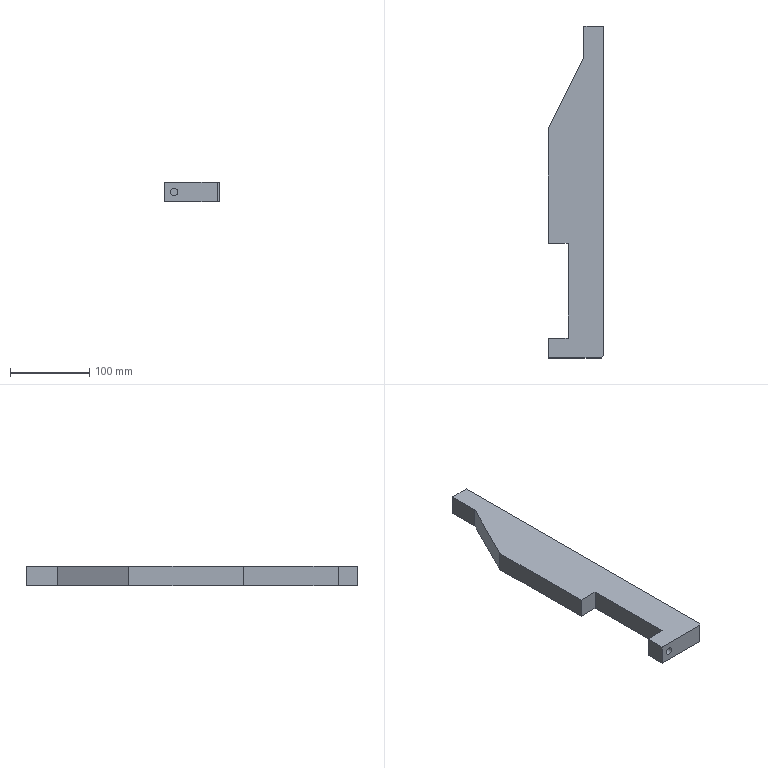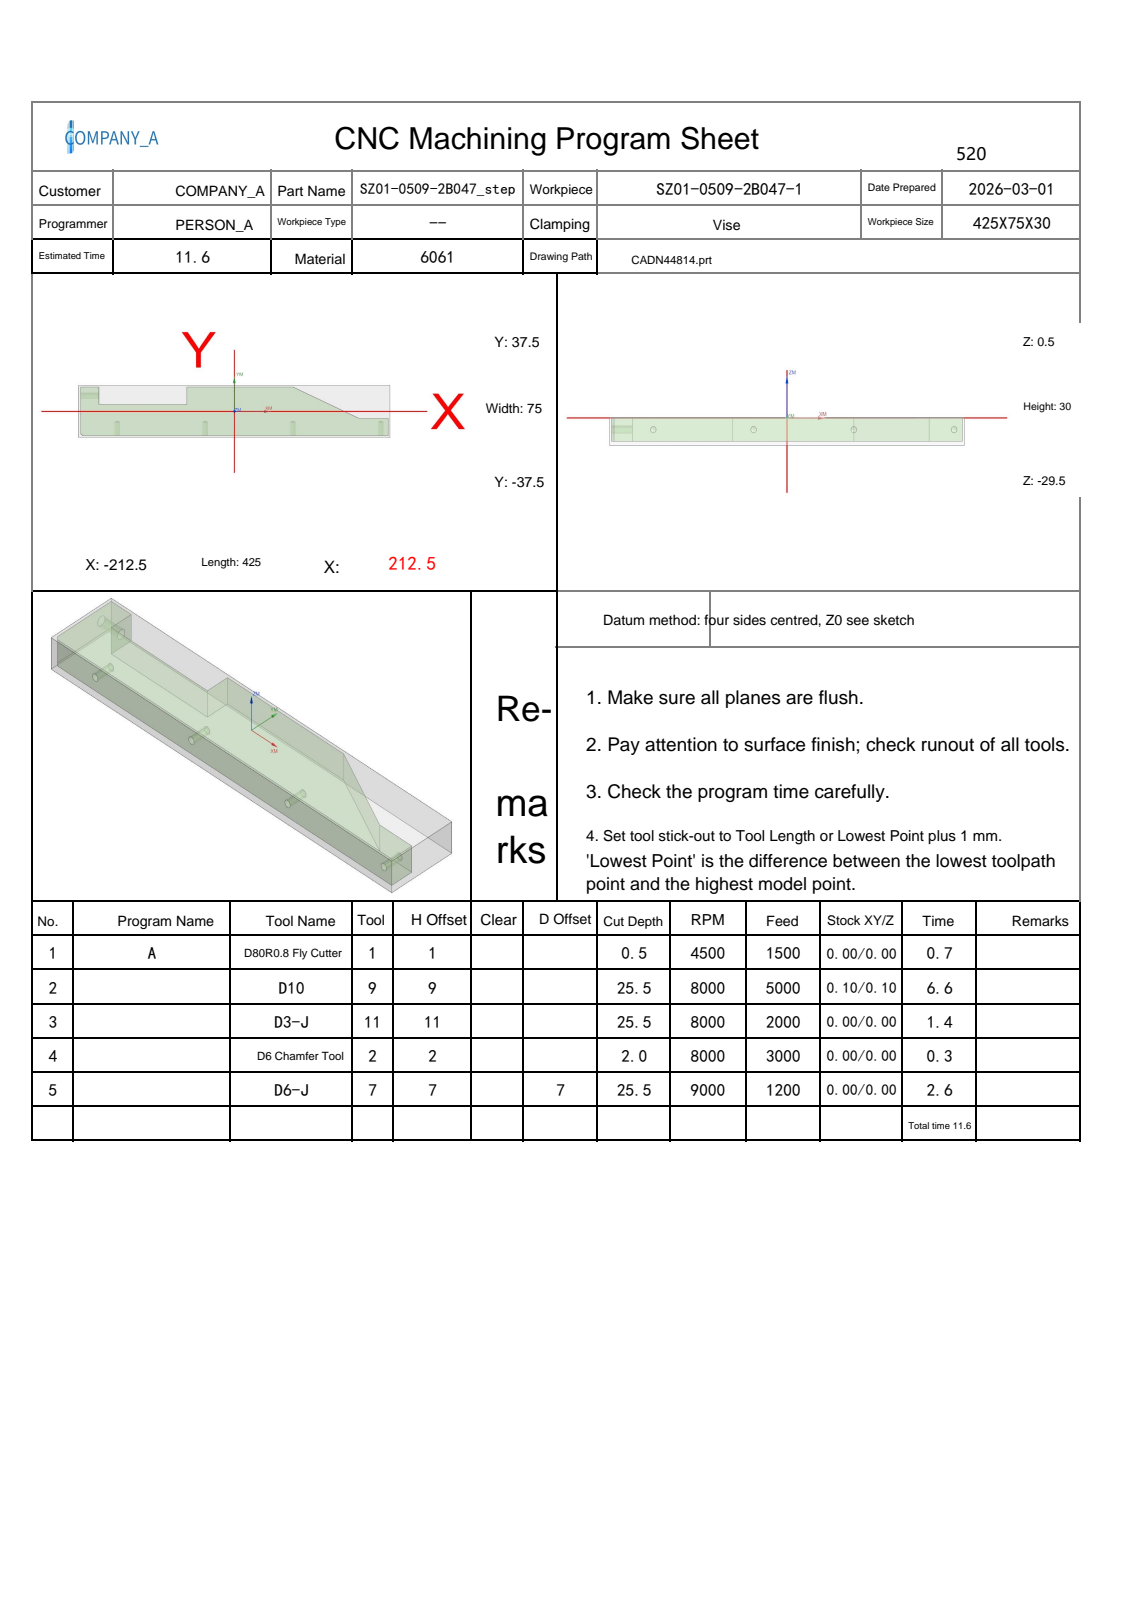NC program | NX | posted by the shop | part box 70 x 420 x 25 mm
Lines 1 to 33 of 10764:
%
O0001
(Machine time: 12.68 MIN)
(===Total Tool:5===)
(T1=D80R0.8 fly cutter D=80.  R=0.8  D-  H01 Z=0.    )
(T9=D10     D=10.  R=0.   D-  H09 Z=-25.  )
(T11=D3-J   D=3.   R=0.   D-  H11 Z=-25.  )
(T2=D6 chamfer tool   D=6.   R=0.   D-  H02 Z=-1.5  )
(T7=D6-J    D=6.   R=0.   D7  H07 Z=-25.  )
G80 G90 G17 G49 G40
G91 G28 Z0
M01
N1 T01 M06
(D80R0.8 fly cutter  D=80. R=0.8 H=01 ce=0.00 di=0.00)
G00 G90 G54 X-255. Y25. M03 S4500
G43 H01 Z50.
M08
Z2.
G01 Z0.0 F1500.
X-250.
X250.
Y-25.
X-250.
X-255.
Z2.
G00 Z50.
G91 G28 Z0.0
M05
M09
G91 G28 Z0.0
M01